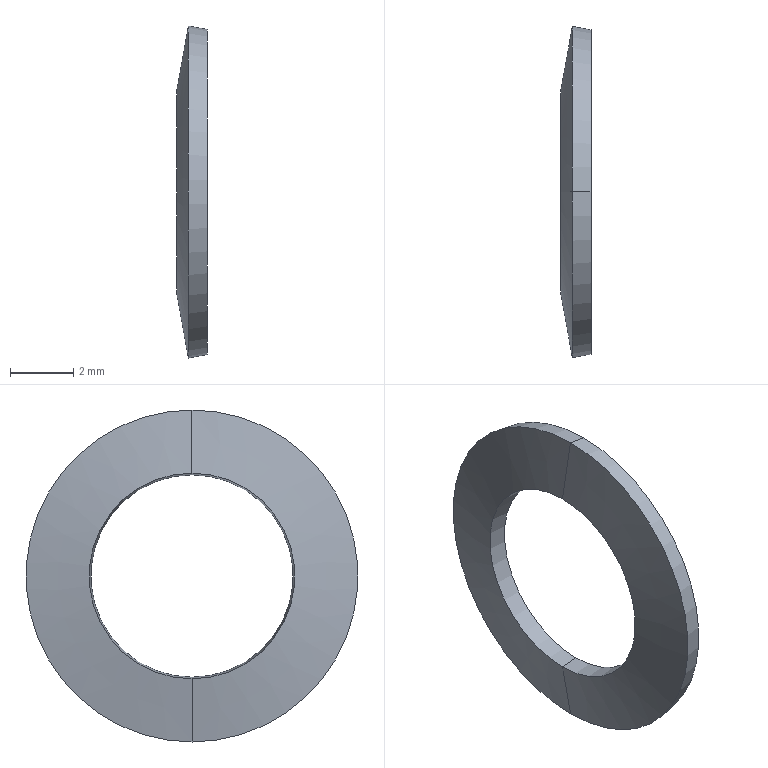Part | STEP file | CW6 Default | 1 solid | 8 faces | box 0.95 x 10.5 x 10.5 mm | volume 31.798 mm3 | cone 8
STEP:
#1=CARTESIAN_POINT('',(0.6,0.,-3.2));
#2=VERTEX_POINT('',#1);
#3=CARTESIAN_POINT('',(0.6,0.,3.2));
#4=VERTEX_POINT('',#3);
#5=CARTESIAN_POINT('',(0.6,0.,0.));
#6=DIRECTION('',(-1.,0.,0.));
#7=DIRECTION('',(0.,0.,1.));
#8=AXIS2_PLACEMENT_3D('',#5,#6,#7);
#9=CIRCLE('',#8,3.2);
#10=EDGE_CURVE('',#2,#4,#9,.T.);
#11=ORIENTED_EDGE('',*,*,#10,.F.);
#12=CARTESIAN_POINT('',(0.,0.,-3.254));
#13=VERTEX_POINT('',#12);
#14=CARTESIAN_POINT('',(0.,0.,-3.254));
#15=DIRECTION('',(-0.996,0.,-0.0889));
#16=VECTOR('',#15,1000.);
#17=LINE('',#14,#16);
#18=EDGE_CURVE('',#2,#13,#17,.T.);
#19=ORIENTED_EDGE('',*,*,#18,.T.);
#20=CARTESIAN_POINT('',(0.,0.,3.254));
#21=VERTEX_POINT('',#20);
#22=CARTESIAN_POINT('',(0.,0.,0.));
#23=DIRECTION('',(-1.,0.,0.));
#24=DIRECTION('',(0.,0.,1.));
#25=AXIS2_PLACEMENT_3D('',#22,#23,#24);
#26=CIRCLE('',#25,3.254);
#27=EDGE_CURVE('',#13,#21,#26,.T.);
#28=ORIENTED_EDGE('',*,*,#27,.T.);
#29=CARTESIAN_POINT('',(0.,0.,3.254));
#30=DIRECTION('',(-0.996,0.,0.0889));
#31=VECTOR('',#30,1000.);
#32=LINE('',#29,#31);
#33=EDGE_CURVE('',#4,#21,#32,.T.);
#34=ORIENTED_EDGE('',*,*,#33,.F.);
#35=EDGE_LOOP('',(#11,#19,#28,#34));
#36=FACE_OUTER_BOUND('',#35,.T.);
#37=CARTESIAN_POINT('',(0.,0.,0.));
#38=DIRECTION('',(-1.,0.,0.));
#39=DIRECTION('',(0.,0.,1.));
#40=AXIS2_PLACEMENT_3D('',#37,#38,#39);
#41=CONICAL_SURFACE('',#40,3.254,0.08902);
#42=ADVANCED_FACE('',(#36),#41,.F.);
#43=ORIENTED_EDGE('',*,*,#10,.T.);
#44=CARTESIAN_POINT('',(0.95,0.,5.145));
#45=VERTEX_POINT('',#44);
#46=CARTESIAN_POINT('',(0.6,0.,3.2));
#47=DIRECTION('',(0.1771,0.,0.9842));
#48=VECTOR('',#47,1000.);
#49=LINE('',#46,#48);
#50=EDGE_CURVE('',#4,#45,#49,.T.);
#51=ORIENTED_EDGE('',*,*,#50,.T.);
#52=CARTESIAN_POINT('',(0.95,0.,-5.145));
#53=VERTEX_POINT('',#52);
#54=CARTESIAN_POINT('',(0.95,0.,0.));
#55=DIRECTION('',(-1.,0.,0.));
#56=DIRECTION('',(0.,0.,1.));
#57=AXIS2_PLACEMENT_3D('',#54,#55,#56);
#58=CIRCLE('',#57,5.145);
#59=EDGE_CURVE('',#53,#45,#58,.T.);
#60=ORIENTED_EDGE('',*,*,#59,.F.);
#61=CARTESIAN_POINT('',(0.6,0.,-3.2));
#62=DIRECTION('',(0.1771,0.,-0.9842));
#63=VECTOR('',#62,1000.);
#64=LINE('',#61,#63);
#65=EDGE_CURVE('',#2,#53,#64,.T.);
#66=ORIENTED_EDGE('',*,*,#65,.F.);
#67=EDGE_LOOP('',(#43,#51,#60,#66));
#68=FACE_OUTER_BOUND('',#67,.T.);
#69=CARTESIAN_POINT('',(0.6,0.,0.));
#70=DIRECTION('',(1.,0.,0.));
#71=DIRECTION('',(0.,0.,-1.));
#72=AXIS2_PLACEMENT_3D('',#69,#70,#71);
#73=CONICAL_SURFACE('',#72,3.2,1.393);
#74=ADVANCED_FACE('',(#68),#73,.F.);
#75=CARTESIAN_POINT('',(0.95,0.,0.));
#76=DIRECTION('',(-1.,0.,0.));
#77=DIRECTION('',(0.,0.,1.));
#78=AXIS2_PLACEMENT_3D('',#75,#76,#77);
#79=CIRCLE('',#78,5.145);
#80=EDGE_CURVE('',#45,#53,#79,.T.);
#81=ORIENTED_EDGE('',*,*,#80,.T.);
#82=CARTESIAN_POINT('',(0.3593,0.,-5.25));
#83=VERTEX_POINT('',#82);
#84=CARTESIAN_POINT('',(0.95,0.,-5.145));
#85=DIRECTION('',(-0.9846,0.,-0.175));
#86=VECTOR('',#85,1000.);
#87=LINE('',#84,#86);
#88=EDGE_CURVE('',#53,#83,#87,.T.);
#89=ORIENTED_EDGE('',*,*,#88,.T.);
#90=CARTESIAN_POINT('',(0.3593,0.,5.25));
#91=VERTEX_POINT('',#90);
#92=CARTESIAN_POINT('',(0.3593,0.,0.));
#93=DIRECTION('',(-1.,0.,0.));
#94=DIRECTION('',(0.,0.,1.));
#95=AXIS2_PLACEMENT_3D('',#92,#93,#94);
#96=CIRCLE('',#95,5.25);
#97=EDGE_CURVE('',#91,#83,#96,.T.);
#98=ORIENTED_EDGE('',*,*,#97,.F.);
#99=CARTESIAN_POINT('',(0.95,0.,5.145));
#100=DIRECTION('',(-0.9846,0.,0.175));
#101=VECTOR('',#100,1000.);
#102=LINE('',#99,#101);
#103=EDGE_CURVE('',#45,#91,#102,.T.);
#104=ORIENTED_EDGE('',*,*,#103,.F.);
#105=EDGE_LOOP('',(#81,#89,#98,#104));
#106=FACE_OUTER_BOUND('',#105,.T.);
#107=CARTESIAN_POINT('',(0.95,0.,0.));
#108=DIRECTION('',(-1.,0.,0.));
#109=DIRECTION('',(0.,0.,1.));
#110=AXIS2_PLACEMENT_3D('',#107,#108,#109);
#111=CONICAL_SURFACE('',#110,5.145,0.1759);
#112=ADVANCED_FACE('',(#106),#111,.T.);
#113=CARTESIAN_POINT('',(0.,0.,0.));
#114=DIRECTION('',(-1.,0.,0.));
#115=DIRECTION('',(0.,0.,1.));
#116=AXIS2_PLACEMENT_3D('',#113,#114,#115);
#117=CIRCLE('',#116,3.254);
#118=EDGE_CURVE('',#21,#13,#117,.T.);
#119=ORIENTED_EDGE('',*,*,#118,.F.);
#120=CARTESIAN_POINT('',(0.3593,0.,5.25));
#121=DIRECTION('',(0.1771,0.,0.9842));
#122=VECTOR('',#121,1000.);
#123=LINE('',#120,#122);
#124=EDGE_CURVE('',#21,#91,#123,.T.);
#125=ORIENTED_EDGE('',*,*,#124,.T.);
#126=ORIENTED_EDGE('',*,*,#97,.T.);
#127=CARTESIAN_POINT('',(0.3593,0.,-5.25));
#128=DIRECTION('',(0.1771,0.,-0.9842));
#129=VECTOR('',#128,1000.);
#130=LINE('',#127,#129);
#131=EDGE_CURVE('',#13,#83,#130,.T.);
#132=ORIENTED_EDGE('',*,*,#131,.F.);
#133=EDGE_LOOP('',(#119,#125,#126,#132));
#134=FACE_OUTER_BOUND('',#133,.T.);
#135=CARTESIAN_POINT('',(0.3593,0.,0.));
#136=DIRECTION('',(1.,0.,0.));
#137=DIRECTION('',(0.,0.,-1.));
#138=AXIS2_PLACEMENT_3D('',#135,#136,#137);
#139=CONICAL_SURFACE('',#138,5.25,1.393);
#140=ADVANCED_FACE('',(#134),#139,.T.);
#141=ORIENTED_EDGE('',*,*,#124,.F.);
#142=ORIENTED_EDGE('',*,*,#27,.F.);
#143=ORIENTED_EDGE('',*,*,#131,.T.);
#144=CARTESIAN_POINT('',(0.3593,0.,0.));
#145=DIRECTION('',(-1.,0.,0.));
#146=DIRECTION('',(0.,0.,1.));
#147=AXIS2_PLACEMENT_3D('',#144,#145,#146);
#148=CIRCLE('',#147,5.25);
#149=EDGE_CURVE('',#83,#91,#148,.T.);
#150=ORIENTED_EDGE('',*,*,#149,.T.);
#151=EDGE_LOOP('',(#141,#142,#143,#150));
#152=FACE_OUTER_BOUND('',#151,.T.);
#153=CARTESIAN_POINT('',(0.3593,0.,0.));
#154=DIRECTION('',(1.,0.,0.));
#155=DIRECTION('',(0.,0.,-1.));
#156=AXIS2_PLACEMENT_3D('',#153,#154,#155);
#157=CONICAL_SURFACE('',#156,5.25,1.393);
#158=ADVANCED_FACE('',(#152),#157,.T.);
#159=ORIENTED_EDGE('',*,*,#88,.F.);
#160=ORIENTED_EDGE('',*,*,#59,.T.);
#161=ORIENTED_EDGE('',*,*,#103,.T.);
#162=ORIENTED_EDGE('',*,*,#149,.F.);
#163=EDGE_LOOP('',(#159,#160,#161,#162));
#164=FACE_OUTER_BOUND('',#163,.T.);
#165=CARTESIAN_POINT('',(0.95,0.,0.));
#166=DIRECTION('',(-1.,0.,0.));
#167=DIRECTION('',(0.,0.,1.));
#168=AXIS2_PLACEMENT_3D('',#165,#166,#167);
#169=CONICAL_SURFACE('',#168,5.145,0.1759);
#170=ADVANCED_FACE('',(#164),#169,.T.);
#171=ORIENTED_EDGE('',*,*,#50,.F.);
#172=CARTESIAN_POINT('',(0.6,0.,0.));
#173=DIRECTION('',(-1.,0.,0.));
#174=DIRECTION('',(0.,0.,1.));
#175=AXIS2_PLACEMENT_3D('',#172,#173,#174);
#176=CIRCLE('',#175,3.2);
#177=EDGE_CURVE('',#4,#2,#176,.T.);
#178=ORIENTED_EDGE('',*,*,#177,.T.);
#179=ORIENTED_EDGE('',*,*,#65,.T.);
#180=ORIENTED_EDGE('',*,*,#80,.F.);
#181=EDGE_LOOP('',(#171,#178,#179,#180));
#182=FACE_OUTER_BOUND('',#181,.T.);
#183=CARTESIAN_POINT('',(0.6,0.,0.));
#184=DIRECTION('',(1.,0.,0.));
#185=DIRECTION('',(0.,0.,-1.));
#186=AXIS2_PLACEMENT_3D('',#183,#184,#185);
#187=CONICAL_SURFACE('',#186,3.2,1.393);
#188=ADVANCED_FACE('',(#182),#187,.F.);
#189=ORIENTED_EDGE('',*,*,#18,.F.);
#190=ORIENTED_EDGE('',*,*,#177,.F.);
#191=ORIENTED_EDGE('',*,*,#33,.T.);
#192=ORIENTED_EDGE('',*,*,#118,.T.);
#193=EDGE_LOOP('',(#189,#190,#191,#192));
#194=FACE_OUTER_BOUND('',#193,.T.);
#195=CARTESIAN_POINT('',(0.,0.,0.));
#196=DIRECTION('',(-1.,0.,0.));
#197=DIRECTION('',(0.,0.,1.));
#198=AXIS2_PLACEMENT_3D('',#195,#196,#197);
#199=CONICAL_SURFACE('',#198,3.254,0.08902);
#200=ADVANCED_FACE('',(#194),#199,.F.);
#201=CLOSED_SHELL('',(#42,#74,#112,#140,#158,#170,#188,#200));
#202=MANIFOLD_SOLID_BREP('',#201);
#203=CARTESIAN_POINT('',(0.,0.,0.));
#204=DIRECTION('',(0.,0.,1.));
#205=DIRECTION('',(1.,0.,0.));
#206=AXIS2_PLACEMENT_3D('',#203,#204,#205);
#207=(LENGTH_UNIT()NAMED_UNIT(*)SI_UNIT(.MILLI.,.METRE.));
#208=UNCERTAINTY_MEASURE_WITH_UNIT(LENGTH_MEASURE(0.00001),#207,'','');
#209=(NAMED_UNIT(*)PLANE_ANGLE_UNIT()SI_UNIT($,.RADIAN.));
#210=(NAMED_UNIT(*)SI_UNIT($,.STERADIAN.)SOLID_ANGLE_UNIT());
#211=(GEOMETRIC_REPRESENTATION_CONTEXT(3)GLOBAL_UNCERTAINTY_ASSIGNED_CONTEXT((#208))GLOBAL_UNIT_ASSIGNED_CONTEXT((#207,#209,#210))REPRESENTATION_CONTEXT('',''));
#212=ADVANCED_BREP_SHAPE_REPRESENTATION('',(#202,#206),#211);